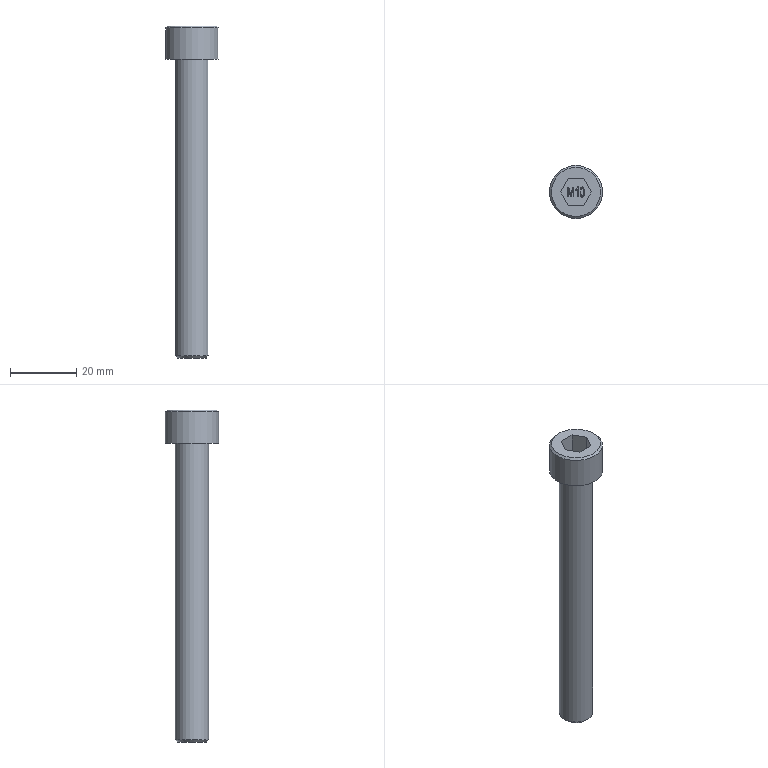Part | STEP file | EM11009000 | 1 solid | 42 faces | box 16 x 16 x 100 mm | volume 8729 mm3 | plane 30 | other 8 | cylinder 2 | cone 2 | commonest cylinder face diameters 10 x1 16 x1